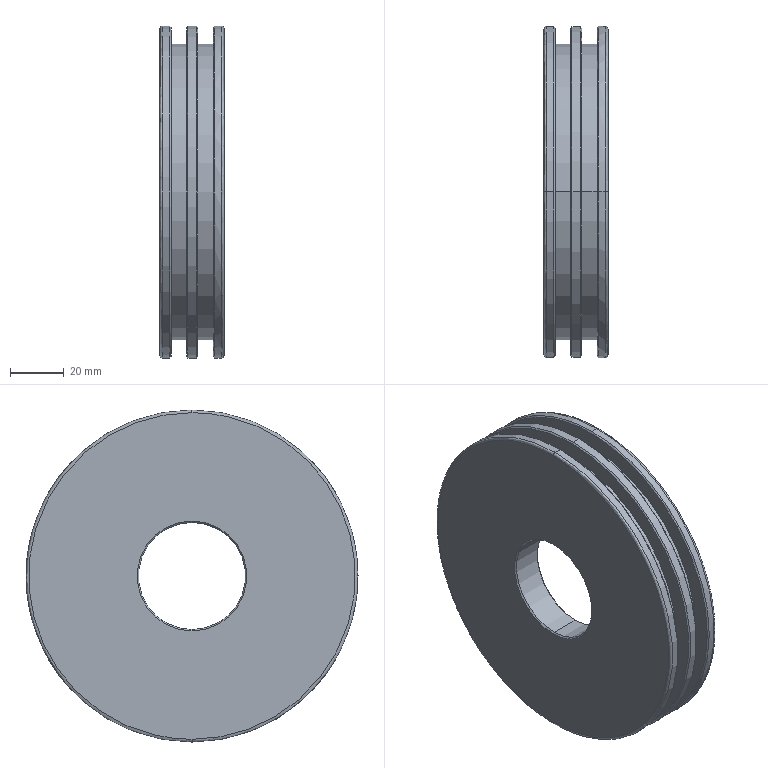Part | SolidWorks | features BaseBody 1 | 1 solid | 39 faces | box 24 x 124 x 124 mm | volume 184707 mm3 | cone 14 | cylinder 14 | plane 7 | spline 4 | commonest cylinder face diameters 124 x6 110.3 x4 40 x2 80 x2